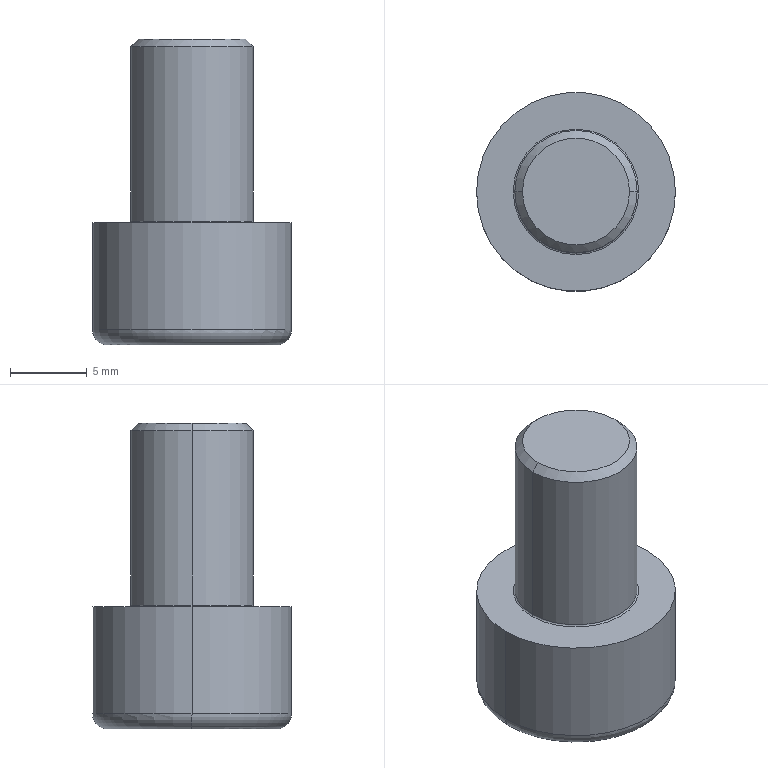Part | SolidWorks | features Fillet 2, ICE 2, Chamfer 1, Extrusion 1 | 1 solid | 20 faces | box 13 x 13 x 20 mm | volume 1529 mm3 | plane 10 | torus 4 | cylinder 4 | cone 2 | commonest cylinder face diameters 8 x2 13 x2
STEP:
#1=CARTESIAN_POINT('',(-5.5,0.,0.));
#2=VERTEX_POINT('',#1);
#3=CARTESIAN_POINT('',(5.5,0.,0.));
#4=VERTEX_POINT('',#3);
#5=CARTESIAN_POINT('',(0.,0.,0.));
#6=DIRECTION('',(0.,0.,-1.));
#7=DIRECTION('',(1.,0.,0.));
#8=AXIS2_PLACEMENT_3D('',#5,#6,#7);
#9=CIRCLE('',#8,5.5);
#10=EDGE_CURVE('',#2,#4,#9,.T.);
#11=ORIENTED_EDGE('',*,*,#10,.F.);
#12=CARTESIAN_POINT('',(-6.5,0.,1.));
#13=VERTEX_POINT('',#12);
#14=CARTESIAN_POINT('',(-5.5,0.,1.));
#15=DIRECTION('',(0.,1.,0.));
#16=DIRECTION('',(-1.,0.,0.));
#17=AXIS2_PLACEMENT_3D('',#14,#15,#16);
#18=CIRCLE('',#17,1.);
#19=EDGE_CURVE('',#2,#13,#18,.T.);
#20=ORIENTED_EDGE('',*,*,#19,.T.);
#21=CARTESIAN_POINT('',(6.5,0.,1.));
#22=VERTEX_POINT('',#21);
#23=CARTESIAN_POINT('',(0.,0.,1.));
#24=DIRECTION('',(0.,0.,1.));
#25=DIRECTION('',(1.,0.,0.));
#26=AXIS2_PLACEMENT_3D('',#23,#24,#25);
#27=CIRCLE('',#26,6.5);
#28=EDGE_CURVE('',#22,#13,#27,.T.);
#29=ORIENTED_EDGE('',*,*,#28,.F.);
#30=CARTESIAN_POINT('',(5.5,0.,1.));
#31=DIRECTION('',(0.,-1.,0.));
#32=DIRECTION('',(0.,0.,-1.));
#33=AXIS2_PLACEMENT_3D('',#30,#31,#32);
#34=CIRCLE('',#33,1.);
#35=EDGE_CURVE('',#4,#22,#34,.T.);
#36=ORIENTED_EDGE('',*,*,#35,.F.);
#37=EDGE_LOOP('',(#11,#20,#29,#36));
#38=FACE_OUTER_BOUND('',#37,.T.);
#39=CARTESIAN_POINT('',(0.,0.,1.));
#40=DIRECTION('',(0.,0.,1.));
#41=DIRECTION('',(1.,0.,0.));
#42=AXIS2_PLACEMENT_3D('',#39,#40,#41);
#43=TOROIDAL_SURFACE('',#42,5.5,1.);
#44=ADVANCED_FACE('',(#38),#43,.T.);
#45=CARTESIAN_POINT('',(3.5,0.,20.));
#46=VERTEX_POINT('',#45);
#47=CARTESIAN_POINT('',(-3.5,0.,20.));
#48=VERTEX_POINT('',#47);
#49=CARTESIAN_POINT('',(0.,0.,20.));
#50=DIRECTION('',(0.,0.,1.));
#51=DIRECTION('',(1.,0.,0.));
#52=AXIS2_PLACEMENT_3D('',#49,#50,#51);
#53=CIRCLE('',#52,3.5);
#54=EDGE_CURVE('',#46,#48,#53,.T.);
#55=ORIENTED_EDGE('',*,*,#54,.F.);
#56=CARTESIAN_POINT('',(4.,0.,19.5));
#57=VERTEX_POINT('',#56);
#58=CARTESIAN_POINT('',(3.5,0.,20.));
#59=DIRECTION('',(0.7071,0.,-0.7071));
#60=VECTOR('',#59,1000.);
#61=LINE('',#58,#60);
#62=EDGE_CURVE('',#46,#57,#61,.T.);
#63=ORIENTED_EDGE('',*,*,#62,.T.);
#64=CARTESIAN_POINT('',(-4.,0.,19.5));
#65=VERTEX_POINT('',#64);
#66=CARTESIAN_POINT('',(0.,0.,19.5));
#67=DIRECTION('',(0.,0.,-1.));
#68=DIRECTION('',(1.,0.,0.));
#69=AXIS2_PLACEMENT_3D('',#66,#67,#68);
#70=CIRCLE('',#69,4.);
#71=EDGE_CURVE('',#65,#57,#70,.T.);
#72=ORIENTED_EDGE('',*,*,#71,.F.);
#73=CARTESIAN_POINT('',(-3.5,0.,20.));
#74=DIRECTION('',(-0.7071,0.,-0.7071));
#75=VECTOR('',#74,1000.);
#76=LINE('',#73,#75);
#77=EDGE_CURVE('',#48,#65,#76,.T.);
#78=ORIENTED_EDGE('',*,*,#77,.F.);
#79=EDGE_LOOP('',(#55,#63,#72,#78));
#80=FACE_OUTER_BOUND('',#79,.T.);
#81=CARTESIAN_POINT('',(0.,0.,20.));
#82=DIRECTION('',(0.,0.,-1.));
#83=DIRECTION('',(-1.,0.,0.));
#84=AXIS2_PLACEMENT_3D('',#81,#82,#83);
#85=CONICAL_SURFACE('',#84,3.5,0.7854);
#86=ADVANCED_FACE('',(#80),#85,.T.);
#87=CARTESIAN_POINT('',(-4.,0.,8.1));
#88=VERTEX_POINT('',#87);
#89=CARTESIAN_POINT('',(4.,0.,8.1));
#90=VERTEX_POINT('',#89);
#91=CARTESIAN_POINT('',(0.,0.,8.1));
#92=DIRECTION('',(0.,0.,1.));
#93=DIRECTION('',(1.,0.,0.));
#94=AXIS2_PLACEMENT_3D('',#91,#92,#93);
#95=CIRCLE('',#94,4.);
#96=EDGE_CURVE('',#88,#90,#95,.T.);
#97=ORIENTED_EDGE('',*,*,#96,.F.);
#98=CARTESIAN_POINT('',(-4.1,0.,8.));
#99=VERTEX_POINT('',#98);
#100=CARTESIAN_POINT('',(-4.1,0.,8.1));
#101=DIRECTION('',(0.,1.,0.));
#102=DIRECTION('',(-1.,0.,0.));
#103=AXIS2_PLACEMENT_3D('',#100,#101,#102);
#104=CIRCLE('',#103,0.1);
#105=EDGE_CURVE('',#88,#99,#104,.T.);
#106=ORIENTED_EDGE('',*,*,#105,.T.);
#107=CARTESIAN_POINT('',(4.1,0.,8.));
#108=VERTEX_POINT('',#107);
#109=CARTESIAN_POINT('',(0.,0.,8.));
#110=DIRECTION('',(0.,0.,-1.));
#111=DIRECTION('',(1.,0.,0.));
#112=AXIS2_PLACEMENT_3D('',#109,#110,#111);
#113=CIRCLE('',#112,4.1);
#114=EDGE_CURVE('',#108,#99,#113,.T.);
#115=ORIENTED_EDGE('',*,*,#114,.F.);
#116=CARTESIAN_POINT('',(4.1,0.,8.1));
#117=DIRECTION('',(0.,-1.,0.));
#118=DIRECTION('',(0.,0.,-1.));
#119=AXIS2_PLACEMENT_3D('',#116,#117,#118);
#120=CIRCLE('',#119,0.1);
#121=EDGE_CURVE('',#90,#108,#120,.T.);
#122=ORIENTED_EDGE('',*,*,#121,.F.);
#123=EDGE_LOOP('',(#97,#106,#115,#122));
#124=FACE_OUTER_BOUND('',#123,.T.);
#125=CARTESIAN_POINT('',(0.,0.,8.1));
#126=DIRECTION('',(0.,0.,1.));
#127=DIRECTION('',(1.,0.,0.));
#128=AXIS2_PLACEMENT_3D('',#125,#126,#127);
#129=TOROIDAL_SURFACE('',#128,4.1,0.1);
#130=ADVANCED_FACE('',(#124),#129,.F.);
#131=ORIENTED_EDGE('',*,*,#71,.T.);
#132=CARTESIAN_POINT('',(4.,0.,20.));
#133=DIRECTION('',(0.,0.,-1.));
#134=VECTOR('',#133,1000.);
#135=LINE('',#132,#134);
#136=EDGE_CURVE('',#57,#90,#135,.T.);
#137=ORIENTED_EDGE('',*,*,#136,.T.);
#138=CARTESIAN_POINT('',(0.,0.,8.1));
#139=DIRECTION('',(0.,0.,1.));
#140=DIRECTION('',(1.,0.,0.));
#141=AXIS2_PLACEMENT_3D('',#138,#139,#140);
#142=CIRCLE('',#141,4.);
#143=EDGE_CURVE('',#90,#88,#142,.T.);
#144=ORIENTED_EDGE('',*,*,#143,.T.);
#145=CARTESIAN_POINT('',(-4.,0.,20.));
#146=DIRECTION('',(0.,0.,-1.));
#147=VECTOR('',#146,1000.);
#148=LINE('',#145,#147);
#149=EDGE_CURVE('',#65,#88,#148,.T.);
#150=ORIENTED_EDGE('',*,*,#149,.F.);
#151=EDGE_LOOP('',(#131,#137,#144,#150));
#152=FACE_OUTER_BOUND('',#151,.T.);
#153=CARTESIAN_POINT('',(0.,0.,20.));
#154=DIRECTION('',(0.,0.,-1.));
#155=DIRECTION('',(-1.,0.,0.));
#156=AXIS2_PLACEMENT_3D('',#153,#154,#155);
#157=CYLINDRICAL_SURFACE('',#156,4.);
#158=ADVANCED_FACE('',(#152),#157,.T.);
#159=CARTESIAN_POINT('',(6.5,0.,8.));
#160=VERTEX_POINT('',#159);
#161=CARTESIAN_POINT('',(-6.5,0.,8.));
#162=VERTEX_POINT('',#161);
#163=CARTESIAN_POINT('',(0.,0.,8.));
#164=DIRECTION('',(0.,0.,1.));
#165=DIRECTION('',(1.,0.,0.));
#166=AXIS2_PLACEMENT_3D('',#163,#164,#165);
#167=CIRCLE('',#166,6.5);
#168=EDGE_CURVE('',#160,#162,#167,.T.);
#169=ORIENTED_EDGE('',*,*,#168,.F.);
#170=CARTESIAN_POINT('',(6.5,0.,8.));
#171=DIRECTION('',(0.,0.,-1.));
#172=VECTOR('',#171,1000.);
#173=LINE('',#170,#172);
#174=EDGE_CURVE('',#160,#22,#173,.T.);
#175=ORIENTED_EDGE('',*,*,#174,.T.);
#176=ORIENTED_EDGE('',*,*,#28,.T.);
#177=CARTESIAN_POINT('',(-6.5,0.,8.));
#178=DIRECTION('',(0.,0.,-1.));
#179=VECTOR('',#178,1000.);
#180=LINE('',#177,#179);
#181=EDGE_CURVE('',#162,#13,#180,.T.);
#182=ORIENTED_EDGE('',*,*,#181,.F.);
#183=EDGE_LOOP('',(#169,#175,#176,#182));
#184=FACE_OUTER_BOUND('',#183,.T.);
#185=CARTESIAN_POINT('',(0.,0.,8.));
#186=DIRECTION('',(0.,0.,-1.));
#187=DIRECTION('',(-1.,0.,0.));
#188=AXIS2_PLACEMENT_3D('',#185,#186,#187);
#189=CYLINDRICAL_SURFACE('',#188,6.5);
#190=ADVANCED_FACE('',(#184),#189,.T.);
#191=ORIENTED_EDGE('',*,*,#174,.F.);
#192=CARTESIAN_POINT('',(0.,0.,8.));
#193=DIRECTION('',(0.,0.,1.));
#194=DIRECTION('',(1.,0.,0.));
#195=AXIS2_PLACEMENT_3D('',#192,#193,#194);
#196=CIRCLE('',#195,6.5);
#197=EDGE_CURVE('',#162,#160,#196,.T.);
#198=ORIENTED_EDGE('',*,*,#197,.F.);
#199=ORIENTED_EDGE('',*,*,#181,.T.);
#200=CARTESIAN_POINT('',(0.,0.,1.));
#201=DIRECTION('',(0.,0.,1.));
#202=DIRECTION('',(1.,0.,0.));
#203=AXIS2_PLACEMENT_3D('',#200,#201,#202);
#204=CIRCLE('',#203,6.5);
#205=EDGE_CURVE('',#13,#22,#204,.T.);
#206=ORIENTED_EDGE('',*,*,#205,.T.);
#207=EDGE_LOOP('',(#191,#198,#199,#206));
#208=FACE_OUTER_BOUND('',#207,.T.);
#209=CARTESIAN_POINT('',(0.,0.,8.));
#210=DIRECTION('',(0.,0.,-1.));
#211=DIRECTION('',(-1.,0.,0.));
#212=AXIS2_PLACEMENT_3D('',#209,#210,#211);
#213=CYLINDRICAL_SURFACE('',#212,6.5);
#214=ADVANCED_FACE('',(#208),#213,.T.);
#215=ORIENTED_EDGE('',*,*,#114,.T.);
#216=CARTESIAN_POINT('',(0.,0.,8.));
#217=DIRECTION('',(0.,0.,-1.));
#218=DIRECTION('',(1.,0.,0.));
#219=AXIS2_PLACEMENT_3D('',#216,#217,#218);
#220=CIRCLE('',#219,4.1);
#221=EDGE_CURVE('',#99,#108,#220,.T.);
#222=ORIENTED_EDGE('',*,*,#221,.T.);
#223=EDGE_LOOP('',(#215,#222));
#224=FACE_BOUND('',#223,.T.);
#225=ORIENTED_EDGE('',*,*,#197,.T.);
#226=ORIENTED_EDGE('',*,*,#168,.T.);
#227=EDGE_LOOP('',(#225,#226));
#228=FACE_OUTER_BOUND('',#227,.T.);
#229=CARTESIAN_POINT('',(0.,0.,8.));
#230=DIRECTION('',(0.,0.,1.));
#231=DIRECTION('',(1.,0.,0.));
#232=AXIS2_PLACEMENT_3D('',#229,#230,#231);
#233=PLANE('',#232);
#234=ADVANCED_FACE('',(#224,#228),#233,.T.);
#235=CARTESIAN_POINT('',(0.,0.,0.));
#236=DIRECTION('',(0.,0.,-1.));
#237=DIRECTION('',(1.,0.,0.));
#238=AXIS2_PLACEMENT_3D('',#235,#236,#237);
#239=CIRCLE('',#238,5.5);
#240=EDGE_CURVE('',#4,#2,#239,.T.);
#241=ORIENTED_EDGE('',*,*,#240,.T.);
#242=ORIENTED_EDGE('',*,*,#10,.T.);
#243=EDGE_LOOP('',(#241,#242));
#244=FACE_OUTER_BOUND('',#243,.T.);
#245=CARTESIAN_POINT('',(-1.732,-3.,0.));
#246=VERTEX_POINT('',#245);
#247=CARTESIAN_POINT('',(-3.464,0.,0.));
#248=VERTEX_POINT('',#247);
#249=CARTESIAN_POINT('',(-1.732,-3.,0.));
#250=DIRECTION('',(-0.5,0.866,0.));
#251=VECTOR('',#250,1000.);
#252=LINE('',#249,#251);
#253=EDGE_CURVE('',#246,#248,#252,.T.);
#254=ORIENTED_EDGE('',*,*,#253,.F.);
#255=CARTESIAN_POINT('',(1.732,-3.,0.));
#256=VERTEX_POINT('',#255);
#257=CARTESIAN_POINT('',(1.732,-3.,0.));
#258=DIRECTION('',(-1.,0.,0.));
#259=VECTOR('',#258,1000.);
#260=LINE('',#257,#259);
#261=EDGE_CURVE('',#256,#246,#260,.T.);
#262=ORIENTED_EDGE('',*,*,#261,.F.);
#263=CARTESIAN_POINT('',(3.464,0.,0.));
#264=VERTEX_POINT('',#263);
#265=CARTESIAN_POINT('',(3.464,0.,0.));
#266=DIRECTION('',(-0.5,-0.866,0.));
#267=VECTOR('',#266,1000.);
#268=LINE('',#265,#267);
#269=EDGE_CURVE('',#264,#256,#268,.T.);
#270=ORIENTED_EDGE('',*,*,#269,.F.);
#271=CARTESIAN_POINT('',(1.732,3.,0.));
#272=VERTEX_POINT('',#271);
#273=CARTESIAN_POINT('',(1.732,3.,0.));
#274=DIRECTION('',(0.5,-0.866,0.));
#275=VECTOR('',#274,1000.);
#276=LINE('',#273,#275);
#277=EDGE_CURVE('',#272,#264,#276,.T.);
#278=ORIENTED_EDGE('',*,*,#277,.F.);
#279=CARTESIAN_POINT('',(-1.732,3.,0.));
#280=VERTEX_POINT('',#279);
#281=CARTESIAN_POINT('',(-1.732,3.,0.));
#282=DIRECTION('',(1.,0.,0.));
#283=VECTOR('',#282,1000.);
#284=LINE('',#281,#283);
#285=EDGE_CURVE('',#280,#272,#284,.T.);
#286=ORIENTED_EDGE('',*,*,#285,.F.);
#287=CARTESIAN_POINT('',(-3.464,0.,0.));
#288=DIRECTION('',(0.5,0.866,0.));
#289=VECTOR('',#288,1000.);
#290=LINE('',#287,#289);
#291=EDGE_CURVE('',#248,#280,#290,.T.);
#292=ORIENTED_EDGE('',*,*,#291,.F.);
#293=EDGE_LOOP('',(#254,#262,#270,#278,#286,#292));
#294=FACE_BOUND('',#293,.T.);
#295=CARTESIAN_POINT('',(0.,0.,0.));
#296=DIRECTION('',(0.,0.,1.));
#297=DIRECTION('',(1.,0.,0.));
#298=AXIS2_PLACEMENT_3D('',#295,#296,#297);
#299=PLANE('',#298);
#300=ADVANCED_FACE('',(#244,#294),#299,.F.);
#301=ORIENTED_EDGE('',*,*,#136,.F.);
#302=CARTESIAN_POINT('',(0.,0.,19.5));
#303=DIRECTION('',(0.,0.,-1.));
#304=DIRECTION('',(1.,0.,0.));
#305=AXIS2_PLACEMENT_3D('',#302,#303,#304);
#306=CIRCLE('',#305,4.);
#307=EDGE_CURVE('',#57,#65,#306,.T.);
#308=ORIENTED_EDGE('',*,*,#307,.T.);
#309=ORIENTED_EDGE('',*,*,#149,.T.);
#310=ORIENTED_EDGE('',*,*,#96,.T.);
#311=EDGE_LOOP('',(#301,#308,#309,#310));
#312=FACE_OUTER_BOUND('',#311,.T.);
#313=CARTESIAN_POINT('',(0.,0.,20.));
#314=DIRECTION('',(0.,0.,-1.));
#315=DIRECTION('',(-1.,0.,0.));
#316=AXIS2_PLACEMENT_3D('',#313,#314,#315);
#317=CYLINDRICAL_SURFACE('',#316,4.);
#318=ADVANCED_FACE('',(#312),#317,.T.);
#319=CARTESIAN_POINT('',(0.,0.,20.));
#320=DIRECTION('',(0.,0.,1.));
#321=DIRECTION('',(1.,0.,0.));
#322=AXIS2_PLACEMENT_3D('',#319,#320,#321);
#323=CIRCLE('',#322,3.5);
#324=EDGE_CURVE('',#48,#46,#323,.T.);
#325=ORIENTED_EDGE('',*,*,#324,.T.);
#326=ORIENTED_EDGE('',*,*,#54,.T.);
#327=EDGE_LOOP('',(#325,#326));
#328=FACE_OUTER_BOUND('',#327,.T.);
#329=CARTESIAN_POINT('',(0.,0.,20.));
#330=DIRECTION('',(0.,0.,1.));
#331=DIRECTION('',(1.,0.,0.));
#332=AXIS2_PLACEMENT_3D('',#329,#330,#331);
#333=PLANE('',#332);
#334=ADVANCED_FACE('',(#328),#333,.T.);
#335=ORIENTED_EDGE('',*,*,#261,.T.);
#336=CARTESIAN_POINT('',(-1.732,-3.,4.));
#337=VERTEX_POINT('',#336);
#338=CARTESIAN_POINT('',(-1.732,-3.,4.));
#339=DIRECTION('',(0.,0.,-1.));
#340=VECTOR('',#339,1000.);
#341=LINE('',#338,#340);
#342=EDGE_CURVE('',#337,#246,#341,.T.);
#343=ORIENTED_EDGE('',*,*,#342,.F.);
#344=CARTESIAN_POINT('',(1.732,-3.,4.));
#345=VERTEX_POINT('',#344);
#346=CARTESIAN_POINT('',(1.732,-3.,4.));
#347=DIRECTION('',(-1.,0.,0.));
#348=VECTOR('',#347,1000.);
#349=LINE('',#346,#348);
#350=EDGE_CURVE('',#345,#337,#349,.T.);
#351=ORIENTED_EDGE('',*,*,#350,.F.);
#352=CARTESIAN_POINT('',(1.732,-3.,4.));
#353=DIRECTION('',(0.,0.,-1.));
#354=VECTOR('',#353,1000.);
#355=LINE('',#352,#354);
#356=EDGE_CURVE('',#345,#256,#355,.T.);
#357=ORIENTED_EDGE('',*,*,#356,.T.);
#358=EDGE_LOOP('',(#335,#343,#351,#357));
#359=FACE_OUTER_BOUND('',#358,.T.);
#360=CARTESIAN_POINT('',(1.732,-3.,4.));
#361=DIRECTION('',(0.,-1.,0.));
#362=DIRECTION('',(0.,0.,-1.));
#363=AXIS2_PLACEMENT_3D('',#360,#361,#362);
#364=PLANE('',#363);
#365=ADVANCED_FACE('',(#359),#364,.F.);
#366=ORIENTED_EDGE('',*,*,#269,.T.);
#367=ORIENTED_EDGE('',*,*,#356,.F.);
#368=CARTESIAN_POINT('',(3.464,0.,4.));
#369=VERTEX_POINT('',#368);
#370=CARTESIAN_POINT('',(3.464,0.,4.));
#371=DIRECTION('',(-0.5,-0.866,0.));
#372=VECTOR('',#371,1000.);
#373=LINE('',#370,#372);
#374=EDGE_CURVE('',#369,#345,#373,.T.);
#375=ORIENTED_EDGE('',*,*,#374,.F.);
#376=CARTESIAN_POINT('',(3.464,0.,4.));
#377=DIRECTION('',(0.,0.,-1.));
#378=VECTOR('',#377,1000.);
#379=LINE('',#376,#378);
#380=EDGE_CURVE('',#369,#264,#379,.T.);
#381=ORIENTED_EDGE('',*,*,#380,.T.);
#382=EDGE_LOOP('',(#366,#367,#375,#381));
#383=FACE_OUTER_BOUND('',#382,.T.);
#384=CARTESIAN_POINT('',(3.464,0.,4.));
#385=DIRECTION('',(0.866,-0.5,0.));
#386=DIRECTION('',(0.5,0.866,0.));
#387=AXIS2_PLACEMENT_3D('',#384,#385,#386);
#388=PLANE('',#387);
#389=ADVANCED_FACE('',(#383),#388,.F.);
#390=ORIENTED_EDGE('',*,*,#277,.T.);
#391=ORIENTED_EDGE('',*,*,#380,.F.);
#392=CARTESIAN_POINT('',(1.732,3.,4.));
#393=VERTEX_POINT('',#392);
#394=CARTESIAN_POINT('',(1.732,3.,4.));
#395=DIRECTION('',(0.5,-0.866,0.));
#396=VECTOR('',#395,1000.);
#397=LINE('',#394,#396);
#398=EDGE_CURVE('',#393,#369,#397,.T.);
#399=ORIENTED_EDGE('',*,*,#398,.F.);
#400=CARTESIAN_POINT('',(1.732,3.,4.));
#401=DIRECTION('',(0.,0.,-1.));
#402=VECTOR('',#401,1000.);
#403=LINE('',#400,#402);
#404=EDGE_CURVE('',#393,#272,#403,.T.);
#405=ORIENTED_EDGE('',*,*,#404,.T.);
#406=EDGE_LOOP('',(#390,#391,#399,#405));
#407=FACE_OUTER_BOUND('',#406,.T.);
#408=CARTESIAN_POINT('',(1.732,3.,4.));
#409=DIRECTION('',(0.866,0.5,0.));
#410=DIRECTION('',(-0.5,0.866,0.));
#411=AXIS2_PLACEMENT_3D('',#408,#409,#410);
#412=PLANE('',#411);
#413=ADVANCED_FACE('',(#407),#412,.F.);
#414=ORIENTED_EDGE('',*,*,#285,.T.);
#415=ORIENTED_EDGE('',*,*,#404,.F.);
#416=CARTESIAN_POINT('',(-1.732,3.,4.));
#417=VERTEX_POINT('',#416);
#418=CARTESIAN_POINT('',(-1.732,3.,4.));
#419=DIRECTION('',(1.,0.,0.));
#420=VECTOR('',#419,1000.);
#421=LINE('',#418,#420);
#422=EDGE_CURVE('',#417,#393,#421,.T.);
#423=ORIENTED_EDGE('',*,*,#422,.F.);
#424=CARTESIAN_POINT('',(-1.732,3.,4.));
#425=DIRECTION('',(0.,0.,-1.));
#426=VECTOR('',#425,1000.);
#427=LINE('',#424,#426);
#428=EDGE_CURVE('',#417,#280,#427,.T.);
#429=ORIENTED_EDGE('',*,*,#428,.T.);
#430=EDGE_LOOP('',(#414,#415,#423,#429));
#431=FACE_OUTER_BOUND('',#430,.T.);
#432=CARTESIAN_POINT('',(-1.732,3.,4.));
#433=DIRECTION('',(0.,1.,0.));
#434=DIRECTION('',(0.,0.,1.));
#435=AXIS2_PLACEMENT_3D('',#432,#433,#434);
#436=PLANE('',#435);
#437=ADVANCED_FACE('',(#431),#436,.F.);
#438=ORIENTED_EDGE('',*,*,#291,.T.);
#439=ORIENTED_EDGE('',*,*,#428,.F.);
#440=CARTESIAN_POINT('',(-3.464,0.,4.));
#441=VERTEX_POINT('',#440);
#442=CARTESIAN_POINT('',(-3.464,0.,4.));
#443=DIRECTION('',(0.5,0.866,0.));
#444=VECTOR('',#443,1000.);
#445=LINE('',#442,#444);
#446=EDGE_CURVE('',#441,#417,#445,.T.);
#447=ORIENTED_EDGE('',*,*,#446,.F.);
#448=CARTESIAN_POINT('',(-3.464,0.,4.));
#449=DIRECTION('',(0.,0.,-1.));
#450=VECTOR('',#449,1000.);
#451=LINE('',#448,#450);
#452=EDGE_CURVE('',#441,#248,#451,.T.);
#453=ORIENTED_EDGE('',*,*,#452,.T.);
#454=EDGE_LOOP('',(#438,#439,#447,#453));
#455=FACE_OUTER_BOUND('',#454,.T.);
#456=CARTESIAN_POINT('',(-3.464,0.,4.));
#457=DIRECTION('',(-0.866,0.5,0.));
#458=DIRECTION('',(-0.5,-0.866,0.));
#459=AXIS2_PLACEMENT_3D('',#456,#457,#458);
#460=PLANE('',#459);
#461=ADVANCED_FACE('',(#455),#460,.F.);
#462=ORIENTED_EDGE('',*,*,#253,.T.);
#463=ORIENTED_EDGE('',*,*,#452,.F.);
#464=CARTESIAN_POINT('',(-1.732,-3.,4.));
#465=DIRECTION('',(-0.5,0.866,0.));
#466=VECTOR('',#465,1000.);
#467=LINE('',#464,#466);
#468=EDGE_CURVE('',#337,#441,#467,.T.);
#469=ORIENTED_EDGE('',*,*,#468,.F.);
#470=ORIENTED_EDGE('',*,*,#342,.T.);
#471=EDGE_LOOP('',(#462,#463,#469,#470));
#472=FACE_OUTER_BOUND('',#471,.T.);
#473=CARTESIAN_POINT('',(-1.732,-3.,4.));
#474=DIRECTION('',(-0.866,-0.5,0.));
#475=DIRECTION('',(0.5,-0.866,0.));
#476=AXIS2_PLACEMENT_3D('',#473,#474,#475);
#477=PLANE('',#476);
#478=ADVANCED_FACE('',(#472),#477,.F.);
#479=ORIENTED_EDGE('',*,*,#350,.T.);
#480=ORIENTED_EDGE('',*,*,#468,.T.);
#481=ORIENTED_EDGE('',*,*,#446,.T.);
#482=ORIENTED_EDGE('',*,*,#422,.T.);
#483=ORIENTED_EDGE('',*,*,#398,.T.);
#484=ORIENTED_EDGE('',*,*,#374,.T.);
#485=EDGE_LOOP('',(#479,#480,#481,#482,#483,#484));
#486=FACE_OUTER_BOUND('',#485,.T.);
#487=CARTESIAN_POINT('',(0.,0.,4.));
#488=DIRECTION('',(0.,0.,-1.));
#489=DIRECTION('',(-1.,0.,0.));
#490=AXIS2_PLACEMENT_3D('',#487,#488,#489);
#491=PLANE('',#490);
#492=ADVANCED_FACE('',(#486),#491,.T.);
#493=ORIENTED_EDGE('',*,*,#105,.F.);
#494=ORIENTED_EDGE('',*,*,#143,.F.);
#495=ORIENTED_EDGE('',*,*,#121,.T.);
#496=ORIENTED_EDGE('',*,*,#221,.F.);
#497=EDGE_LOOP('',(#493,#494,#495,#496));
#498=FACE_OUTER_BOUND('',#497,.T.);
#499=CARTESIAN_POINT('',(0.,0.,8.1));
#500=DIRECTION('',(0.,0.,1.));
#501=DIRECTION('',(1.,0.,0.));
#502=AXIS2_PLACEMENT_3D('',#499,#500,#501);
#503=TOROIDAL_SURFACE('',#502,4.1,0.1);
#504=ADVANCED_FACE('',(#498),#503,.F.);
#505=ORIENTED_EDGE('',*,*,#62,.F.);
#506=ORIENTED_EDGE('',*,*,#324,.F.);
#507=ORIENTED_EDGE('',*,*,#77,.T.);
#508=ORIENTED_EDGE('',*,*,#307,.F.);
#509=EDGE_LOOP('',(#505,#506,#507,#508));
#510=FACE_OUTER_BOUND('',#509,.T.);
#511=CARTESIAN_POINT('',(0.,0.,20.));
#512=DIRECTION('',(0.,0.,-1.));
#513=DIRECTION('',(-1.,0.,0.));
#514=AXIS2_PLACEMENT_3D('',#511,#512,#513);
#515=CONICAL_SURFACE('',#514,3.5,0.7854);
#516=ADVANCED_FACE('',(#510),#515,.T.);
#517=ORIENTED_EDGE('',*,*,#19,.F.);
#518=ORIENTED_EDGE('',*,*,#240,.F.);
#519=ORIENTED_EDGE('',*,*,#35,.T.);
#520=ORIENTED_EDGE('',*,*,#205,.F.);
#521=EDGE_LOOP('',(#517,#518,#519,#520));
#522=FACE_OUTER_BOUND('',#521,.T.);
#523=CARTESIAN_POINT('',(0.,0.,1.));
#524=DIRECTION('',(0.,0.,1.));
#525=DIRECTION('',(1.,0.,0.));
#526=AXIS2_PLACEMENT_3D('',#523,#524,#525);
#527=TOROIDAL_SURFACE('',#526,5.5,1.);
#528=ADVANCED_FACE('',(#522),#527,.T.);
#529=CLOSED_SHELL('',(#44,#86,#130,#158,#190,#214,#234,#300,#318,#334,#365,#389,#413,#437,#461,#478,#492,#504,#516,#528));
#530=MANIFOLD_SOLID_BREP('',#529);
#531=CARTESIAN_POINT('',(0.,0.,0.));
#532=DIRECTION('',(0.,0.,1.));
#533=DIRECTION('',(1.,0.,0.));
#534=AXIS2_PLACEMENT_3D('',#531,#532,#533);
#535=(LENGTH_UNIT()NAMED_UNIT(*)SI_UNIT(.MILLI.,.METRE.));
#536=UNCERTAINTY_MEASURE_WITH_UNIT(LENGTH_MEASURE(0.00001),#535,'','');
#537=(NAMED_UNIT(*)PLANE_ANGLE_UNIT()SI_UNIT($,.RADIAN.));
#538=(NAMED_UNIT(*)SI_UNIT($,.STERADIAN.)SOLID_ANGLE_UNIT());
#539=(GEOMETRIC_REPRESENTATION_CONTEXT(3)GLOBAL_UNCERTAINTY_ASSIGNED_CONTEXT((#536))GLOBAL_UNIT_ASSIGNED_CONTEXT((#535,#537,#538))REPRESENTATION_CONTEXT('',''));
#540=ADVANCED_BREP_SHAPE_REPRESENTATION('',(#530,#534),#539);